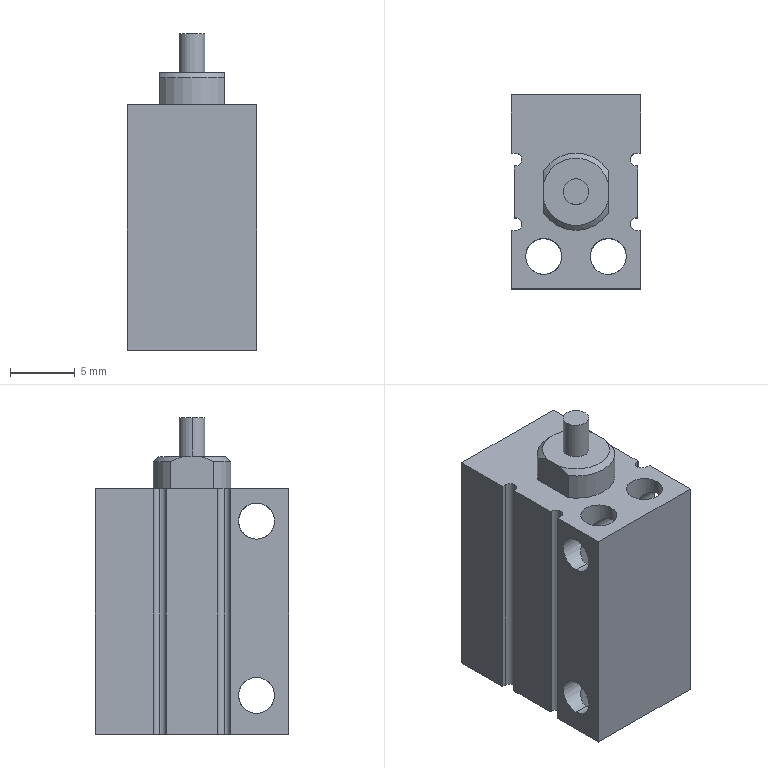Part | NX | features BREP 2 | 2 solids | 80 faces | box 10 x 15 x 24.5 mm | volume 2449 mm3 | cylinder 44 | plane 26 | cone 10 | commonest cylinder face diameters 2.8 x24 1 x6 2 x4 2.459 x4 4 x4 6 x2